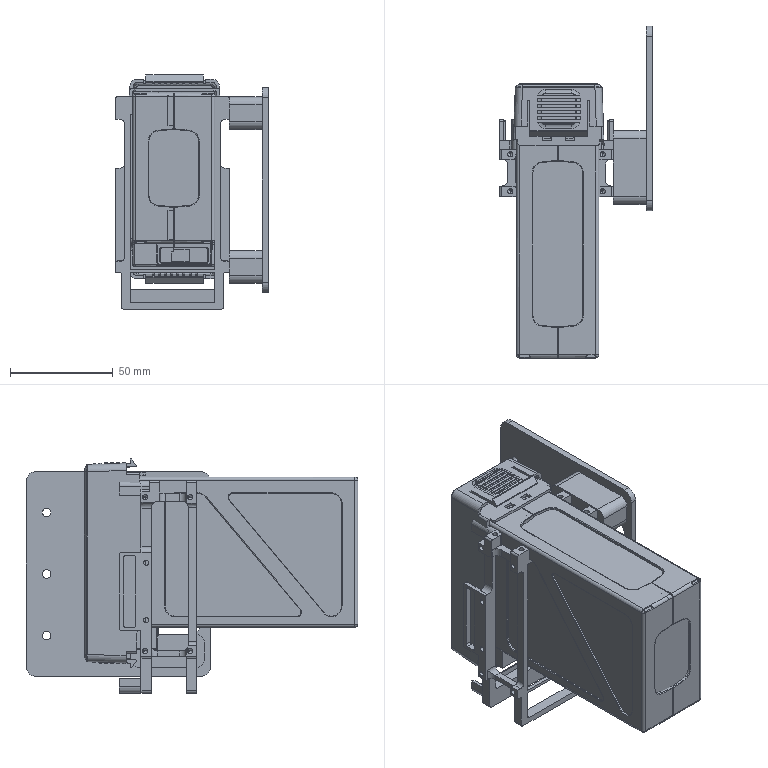Part | SolidWorks | 8 solids | 1683 faces | box 74.4 x 161.725 x 114.085 mm | volume 454834 mm3 | plane 960 | cylinder 477 | spline 180 | cone 53 | torus 13 | commonest cylinder face diameters 1 x85 2 x73 0.6 x66 2.5 x40 6 x40 10 x34